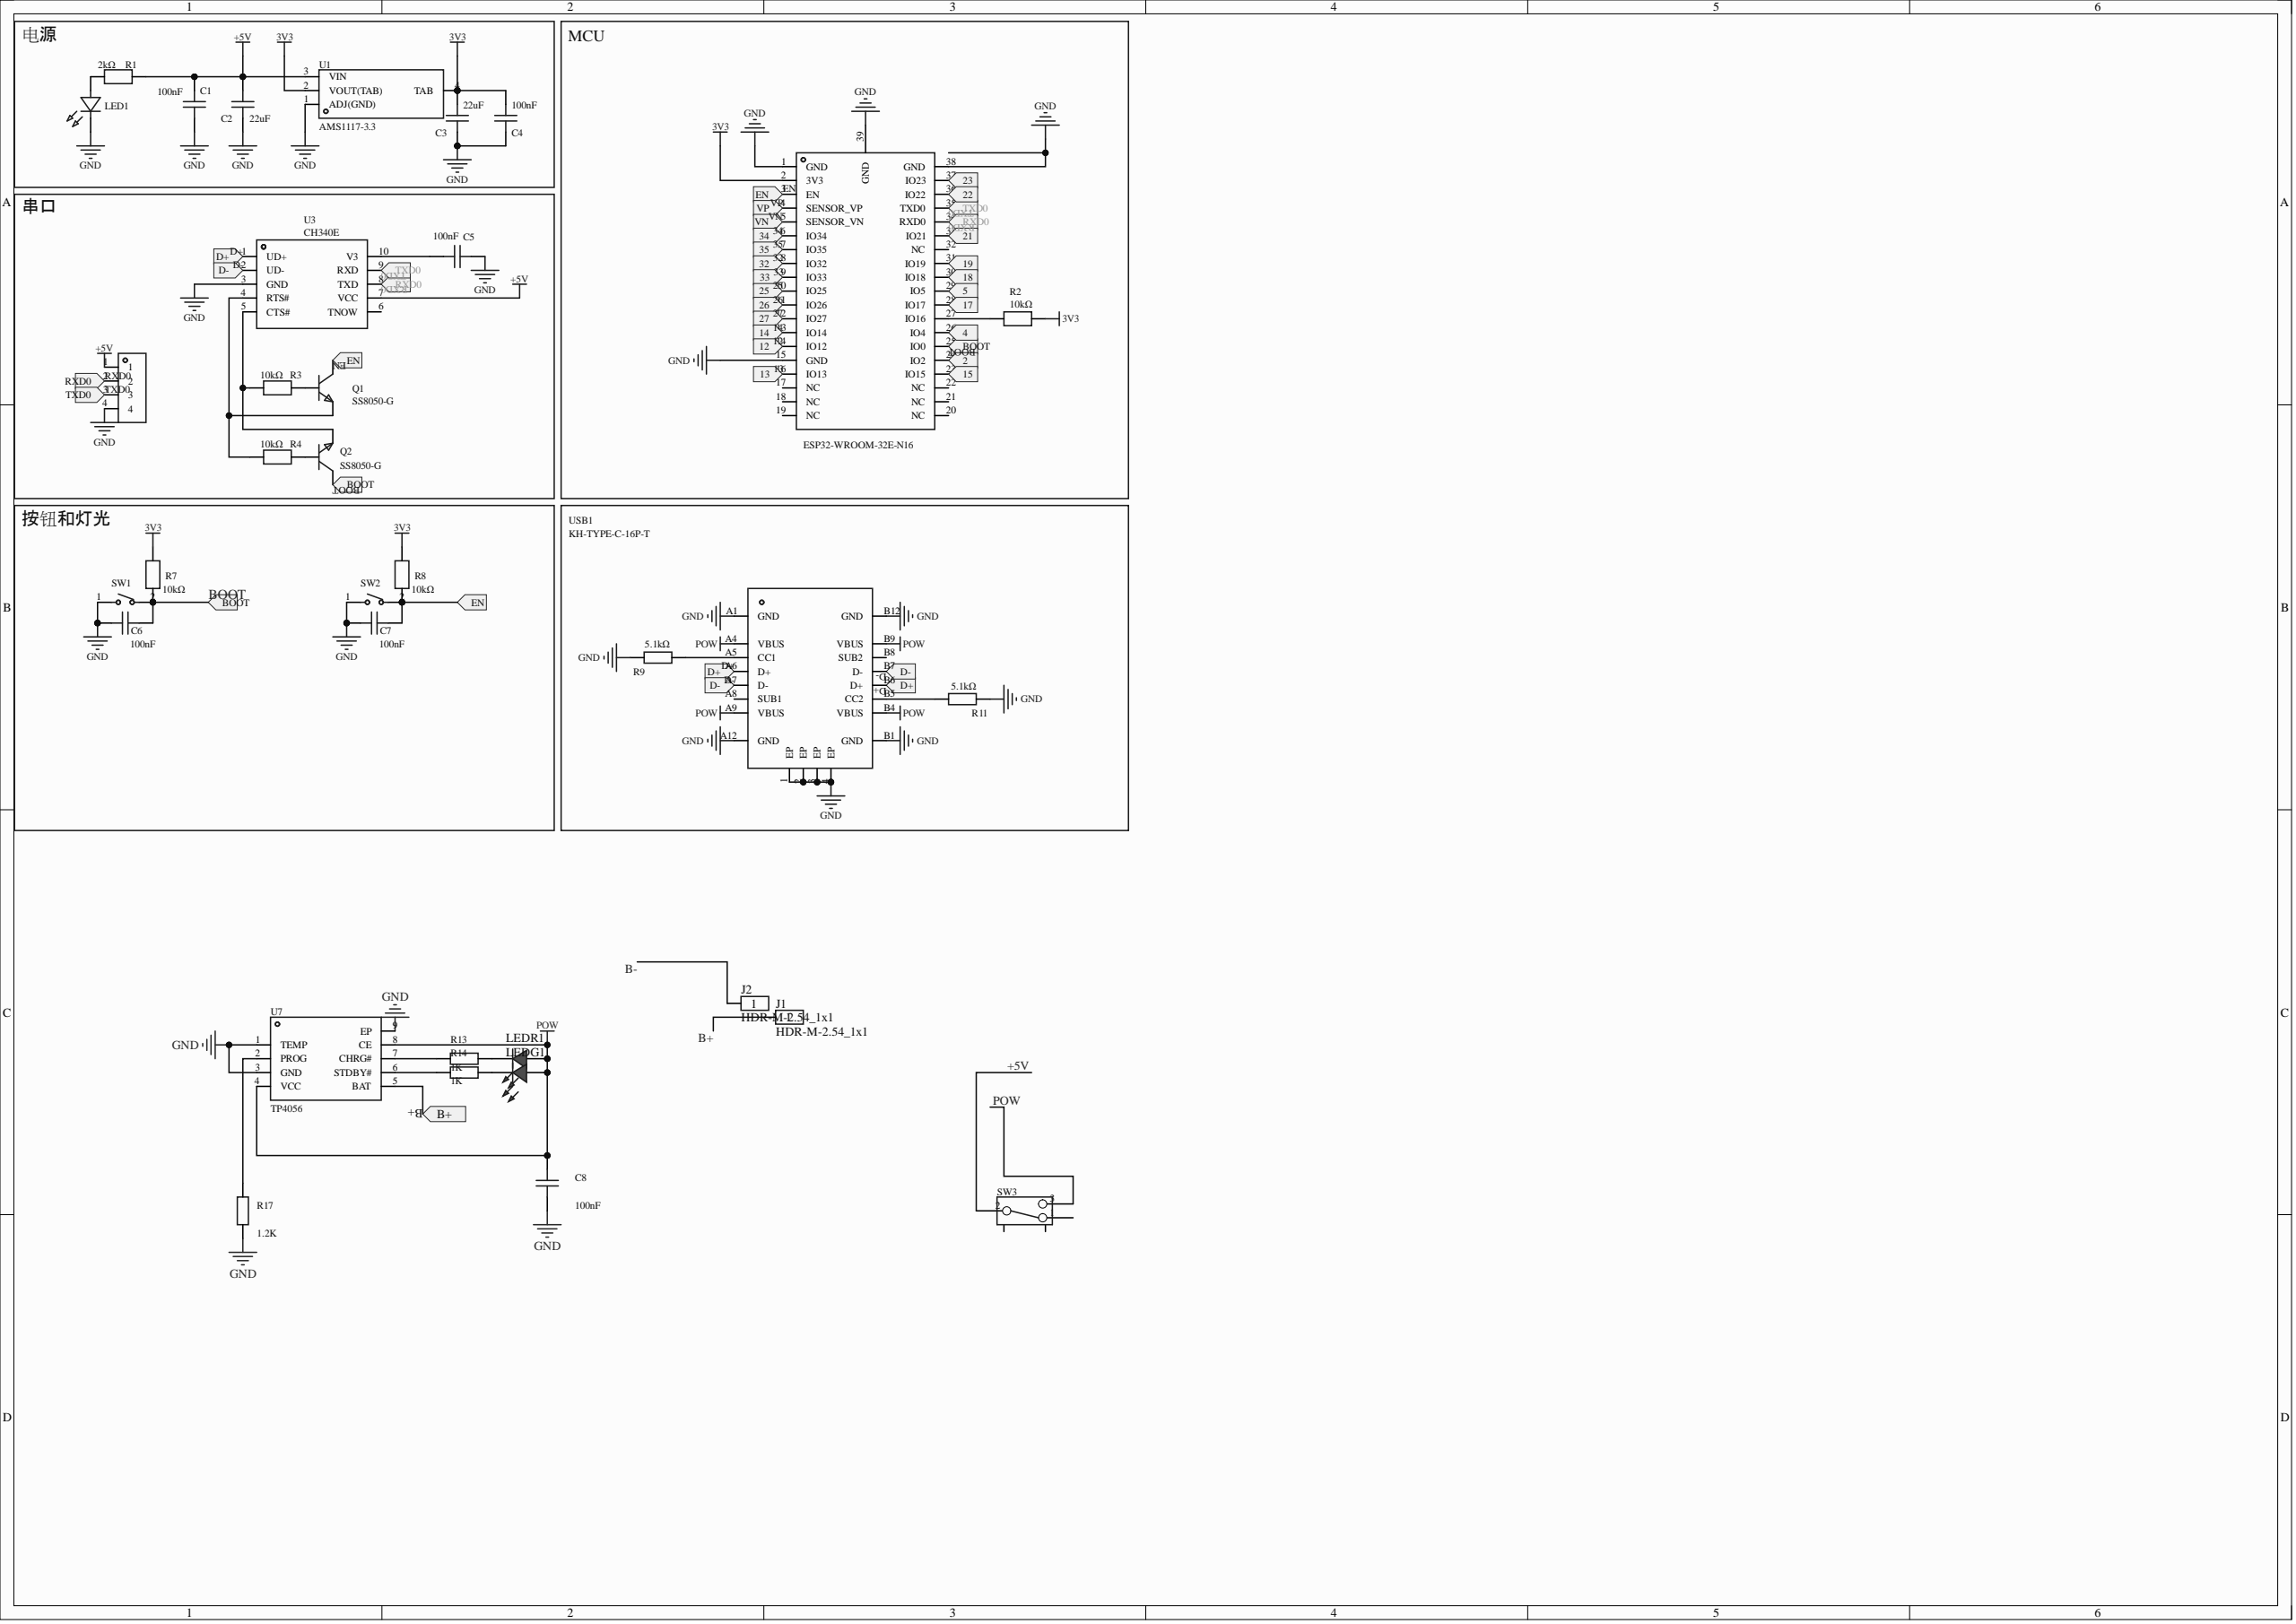Circuit board | Altium Designer | 35 parts | 25 nets
Bill of materials:
Comment,Description,Designator,Footprint,LibRef,Quantity
"100nF","容值:100nF;精度:±20%;额定电压:16V;材质(温度系数):X5R;","C1, C4, C5, C6, C7","C0402","C1005X5R104METS","5"
"22uF","容值:22uF;精度:±20%;额定电压:10V;材质(温度系数):X5R;","C2, C3","C0603","HGC0603R5226M100NTHJ","2"
"100nF","","C8","C0603","CAP_0603","1"
"HDR-M-2.54_1x1","","J1, J2","HDR-M-2.54_1X1","HDR-M-2.54_1x1","2"
"2.54-1*4","插针结构:1x4P;间距:2.54mm;排数:单排;总PIN位数:4P;","J3","HDR-TH_4P-P2.54-V-M-1","2.54-1*4","1"
"XL-1608SURC-06","发光颜色:红色;功率:55mW;正向电流:25mA;主波长:617nm~621nm;透镜颜色:无色透明透镜;色温:-;发光角度:120°;载带方式:正贴;工作温度:-30℃~+85℃;","LED1","LED0603-RD_RED","XL-1608SURC-06","1"
"","","LEDG1, LEDR1","LED_0603","LED_0603-R","2"
"SS8050-G","晶体管类型:NPN;集电极电流(Ic):1.5A;集射极击穿电压(Vceo):25V;功率(Pd):300mW;直流电流增益(hFE@Ic,Vce):200@100mA,1V;","Q1, Q2","SOT-23-3_L2.9-W1.3-P1.90-LS2.4-BR","SS8050-G","2"
"2kΩ","","R1","R0402","SC0402F2001F2ANRH","1"
"10kΩ","","R2, R3, R4, R7, R8","R0402","RCA0210KJLF","5"
"5.1kΩ","","R9, R11","R0201","RTT01512JTH","2"
"1K","","R13, R14","R0603","Res_0603","2"
"1.2K","","R17","R0603","Res_0603","1"
"TSB008A2530A","按钮形状:矩形按钮;作用力:3N;安装方式:立贴;开关长度:6mm;开关宽度:3.5mm;开关高度:2.5mm;触点电流:50mA;额定电压(AC):-;额定电压(DC):12V;机械寿命:-;","SW1, SW2","SW-SMD_L6.0-W3.5-LS8.0","TSB008A2530A","2"
"","","SW3","拨动开关_侧","拨动开关_侧","1"
"AMS1117-3.3","输出类型:固定;最大输入电压:12V;输出电压:3.3V;最大输出电流:1A;电源纹波抑制比(PSRR):60dB@(120Hz);输出极性:正极;","U1","SOT-223-4_L6.5-W3.5-P2.30-LS7.0-BR","AMS1117-3.3_C347222","1"
"ESP32-WROOM-32E-N16","ESP32-WROOM-32E 集成 ESP32-D0WD-V3 芯片，具有高稳定性和安全性能。","U2","WIFI-SMD_ESP32-WROOM-32E","ESP32-WROOM-32E-N16_C701343","1"
"CH340E","应用功能:收发器;接口协议:USB 2.0;数据速率:2Mbps;","U3","MSOP-10_L3.0-W3.0-P0.50-LS5.0-BL","CH340E","1"
"TP4056","","U7","ESOP-8_L4.9-W3.9-P1.27-LS6.0-BL-EP","TP4056_C725790","1"
"KH-TYPE-C-16P-T","连接器类型:Type-C;标准:-;公母:母;端口数量:1;触点数量:16P;安装方式:卧贴;额定电流 - 电源:500mA;工作温度范围:-30℃~+80℃;","USB1","USB-C-SMD_KH-TYPE-C-16P","KH-TYPE-C-16P-T","1"
Netlist (Protel format):
[
C1
C0402
100nF



]
[
C2
C0603
22uF



]
[
C3
C0603
22uF



]
[
C4
C0402
100nF



]
[
C5
C0402
100nF



]
[
C6
C0402
100nF



]
[
C7
C0402
100nF



]
[
C8
C0603
100nF



]
[
J1
HDR-M-2.54_1X1
HDR-M-2.54_1x1



]
[
J2
HDR-M-2.54_1X1
HDR-M-2.54_1x1



]
[
J3
HDR-TH_4P-P2.54-V-M-1
2.54-1*4



]
[
LED1
LED0603-RD_RED
XL-1608SURC-06



]
[
LEDG1
LED_0603




]
[
LEDR1
LED_0603




]
[
Q1
SOT-23-3_L2.9-W1.3-P1.90-LS2.4-BR
SS8050-G



]
[
Q2
SOT-23-3_L2.9-W1.3-P1.90-LS2.4-BR
SS8050-G



]
[
R1
R0402
2kΩ



]
[
R2
R0402
10kΩ



]
[
R3
R0402
10kΩ



]
[
R4
R0402
10kΩ



]
[
R7
R0402
10kΩ



]
[
R8
R0402
10kΩ



]
[
R9
R0201
5.1kΩ



]
[
R11
R0201
5.1kΩ



]
[
R13
R0603
1K



]
[
R14
R0603
1K



]
[
R17
R0603
1.2K



]
[
SW1
SW-SMD_L6.0-W3.5-LS8.0
TSB008A2530A



]
[
SW2
SW-SMD_L6.0-W3.5-LS8.0
TSB008A2530A



]
[
SW3
拨动开关_侧




]
[
U1
SOT-223-4_L6.5-W3.5-P2.30-LS7.0-BR
AMS1117-3.3



]
[
U2
WIFI-SMD_ESP32-WROOM-32E
ESP32-WROOM-32E-N16



]
[
U3
MSOP-10_L3.0-W3.0-P0.50-LS5.0-BL
CH340E



]
[
U7
ESOP-8_L4.9-W3.9-P1.27-LS6.0-BL-EP
TP4056



]
[
USB1
USB-C-SMD_KH-TYPE-C-16P
KH-TYPE-C-16P-T



]
(
TXD0
J3-3
U2-35
U3-9
)
(
RXD0
J3-2
U2-34
U3-8
)
(
POW
C8-2
LEDG1-2
LEDR1-2
SW3-3
U7-4
U7-8
USB1-A4
USB1-A9
USB1-B4
USB1-B9
)
(
NetR17_2
R17-2
U7-2
)
(
NetR14_1
R14-1
U7-6
)
(
NetR13_1
R13-1
U7-7
)
(
NetR11_1
R11-1
USB1-B5
)
(
NetR9_2
R9-2
USB1-A5
)
(
NetR2_1
R2-1
U2-27
)
(
NetQ2_2
Q2-2
R3-1
U3-5
)
(
NetQ2_1
Q2-1
R4-2
)
(
NetQ1_2
Q1-2
R4-1
U3-4
)
(
NetQ1_1
Q1-1
R3-2
)
(
NetLEDR1_1
LEDR1-1
R13-2
)
(
NetLEDG1_1
LEDG1-1
R14-2
)
(
NetLED1_2
LED1-2
R1-1
)
(
NetC5_2
C5-2
U3-10
)
(
GND
C1-1
C2-2
C3-2
C4-1
C5-1
C6-2
C7-2
C8-1
J3-4
LED1-1
R9-1
R11-2
R17-1
SW1-1
SW2-1
U1-1
U2-1
U2-15
U2-38
U2-39
U3-3
U7-1
U7-3
U7-9
USB1-1
USB1-2
USB1-3
USB1-4
USB1-A1
USB1-A12
USB1-B1
USB1-B12
)
(
EN
C7-1
Q1-3
R8-2
SW2-2
U2-3
)
(
D-
U3-2
USB1-A7
USB1-B7
)
(
D+
U3-1
USB1-A6
USB1-B6
)
(
BOOT
C6-1
Q2-3
R7-2
SW1-2
U2-25
)
(
B+
J1-1
U7-5
)
(
+5V
C1-2
C2-1
J3-1
R1-2
SW3-2
U1-3
U3-7
)
(
3V3
C3-1
C4-2
R2-2
R7-1
R8-1
U1-2
U1-4
U2-2
)